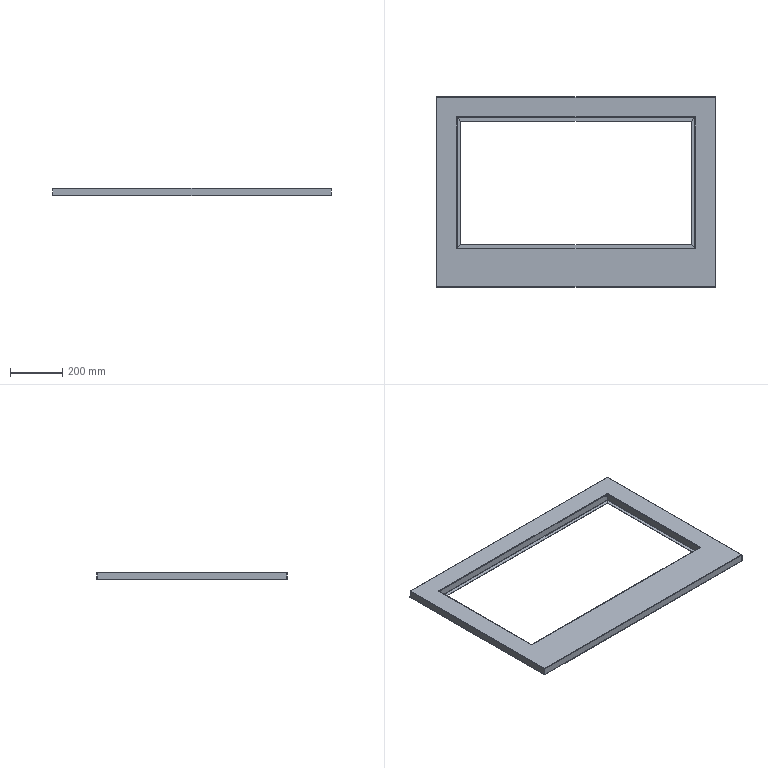Part | SolidWorks | features EdgeFlange 4, FlatPattern 1, HoleWzd 1, ICE 1, SMBaseFlange 1, SheetMetal 1 | 1 solid | 146 faces | box 1070 x 730 x 30 mm | volume 905404 mm3 | plane 74 | cylinder 40 | spline 32 | commonest cylinder face diameters 1 x16 4 x16 5 x8